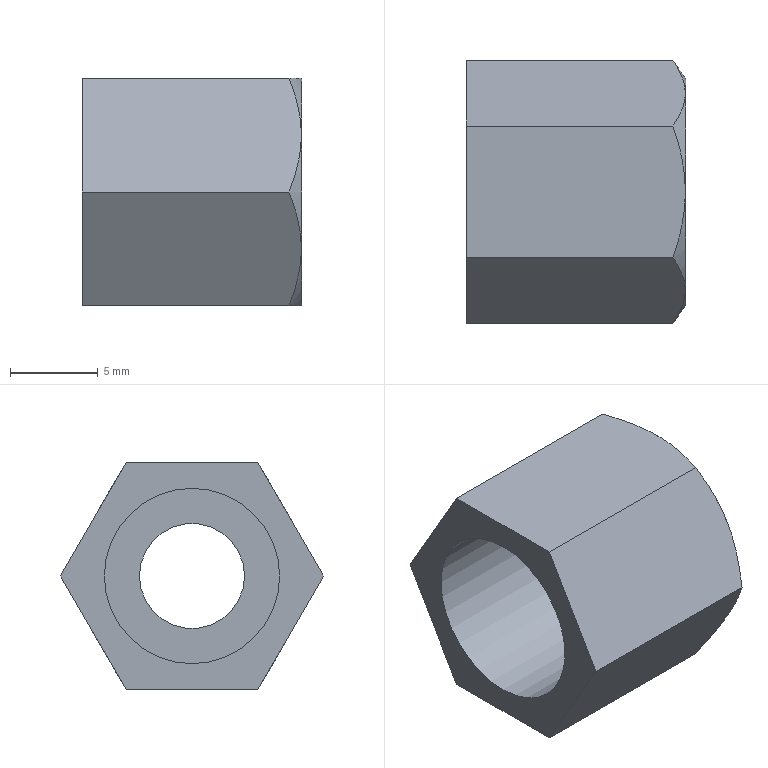Part | STEP file | 1-55.5 | 2 solids | 16 faces | box 12.5 x 15.011 x 13 mm | volume 1071 mm3 | plane 11 | cylinder 4 | cone 1 | commonest cylinder face diameters 6 x2 10 x2
STEP:
#1=CARTESIAN_POINT('',(0.,0.,0.));
#2=DIRECTION('',(0.,0.,1.));
#3=DIRECTION('',(1.,0.,0.));
#4=AXIS2_PLACEMENT_3D('',#1,#2,#3);
#5=CARTESIAN_POINT('',(0.,-3.753,6.5));
#6=VERTEX_POINT('',#5);
#7=CARTESIAN_POINT('',(0.,3.753,6.5));
#8=VERTEX_POINT('',#7);
#9=CARTESIAN_POINT('',(0.,-3.753,6.5));
#10=DIRECTION('',(0.,1.,0.));
#11=VECTOR('',#10,1.);
#12=LINE('',#9,#11);
#13=CARTESIAN_POINT('',(0.,0.,1.006));
#14=DIRECTION('',(-1.,0.,0.));
#15=DIRECTION('',(0.,0.,1.));
#16=AXIS2_PLACEMENT_3D('',#13,#14,#15);
#17=PLANE('',#16);
#18=CARTESIAN_POINT('',(5.494,-3.753));
#19=DIRECTION('',(0.,1.));
#20=VECTOR('',#19,1.);
#21=LINE('',#18,#20);
#22=(GEOMETRIC_REPRESENTATION_CONTEXT(2)PARAMETRIC_REPRESENTATION_CONTEXT()REPRESENTATION_CONTEXT('',''));
#23=DEFINITIONAL_REPRESENTATION('',(#21),#22);
#24=PCURVE('',#17,#23);
#25=CARTESIAN_POINT('',(6.25,0.,6.5));
#26=DIRECTION('',(0.,0.,-1.));
#27=DIRECTION('',(0.,1.,0.));
#28=AXIS2_PLACEMENT_3D('',#25,#26,#27);
#29=PLANE('',#28);
#30=CARTESIAN_POINT('',(-3.753,-6.25));
#31=DIRECTION('',(1.,0.));
#32=VECTOR('',#31,1.);
#33=LINE('',#30,#32);
#34=(GEOMETRIC_REPRESENTATION_CONTEXT(2)PARAMETRIC_REPRESENTATION_CONTEXT()REPRESENTATION_CONTEXT('',''));
#35=DEFINITIONAL_REPRESENTATION('',(#33),#34);
#36=PCURVE('',#29,#35);
#37=SURFACE_CURVE('',#12,(#24,#36),.PCURVE_S1.);
#38=EDGE_CURVE('',#6,#8,#37,.T.);
#39=ORIENTED_EDGE('',*,*,#38,.T.);
#40=CARTESIAN_POINT('',(0.,7.506,0.));
#41=VERTEX_POINT('',#40);
#42=CARTESIAN_POINT('',(0.,3.753,6.5));
#43=DIRECTION('',(0.,0.5,-0.866));
#44=VECTOR('',#43,1.);
#45=LINE('',#42,#44);
#46=CARTESIAN_POINT('',(5.494,3.753));
#47=DIRECTION('',(-0.866,0.5));
#48=VECTOR('',#47,1.);
#49=LINE('',#46,#48);
#50=(GEOMETRIC_REPRESENTATION_CONTEXT(2)PARAMETRIC_REPRESENTATION_CONTEXT()REPRESENTATION_CONTEXT('',''));
#51=DEFINITIONAL_REPRESENTATION('',(#49),#50);
#52=PCURVE('',#17,#51);
#53=CARTESIAN_POINT('',(6.25,5.629,3.25));
#54=DIRECTION('',(0.,-0.866,-0.5));
#55=DIRECTION('',(0.,0.5,-0.866));
#56=AXIS2_PLACEMENT_3D('',#53,#54,#55);
#57=PLANE('',#56);
#58=CARTESIAN_POINT('',(-3.753,-6.25));
#59=DIRECTION('',(1.,0.));
#60=VECTOR('',#59,1.);
#61=LINE('',#58,#60);
#62=(GEOMETRIC_REPRESENTATION_CONTEXT(2)PARAMETRIC_REPRESENTATION_CONTEXT()REPRESENTATION_CONTEXT('',''));
#63=DEFINITIONAL_REPRESENTATION('',(#61),#62);
#64=PCURVE('',#57,#63);
#65=SURFACE_CURVE('',#45,(#52,#64),.PCURVE_S1.);
#66=EDGE_CURVE('',#8,#41,#65,.T.);
#67=ORIENTED_EDGE('',*,*,#66,.T.);
#68=CARTESIAN_POINT('',(0.,3.753,-6.5));
#69=VERTEX_POINT('',#68);
#70=CARTESIAN_POINT('',(0.,7.506,0.));
#71=DIRECTION('',(0.,-0.5,-0.866));
#72=VECTOR('',#71,1.);
#73=LINE('',#70,#72);
#74=CARTESIAN_POINT('',(-1.006,7.506));
#75=DIRECTION('',(-0.866,-0.5));
#76=VECTOR('',#75,1.);
#77=LINE('',#74,#76);
#78=(GEOMETRIC_REPRESENTATION_CONTEXT(2)PARAMETRIC_REPRESENTATION_CONTEXT()REPRESENTATION_CONTEXT('',''));
#79=DEFINITIONAL_REPRESENTATION('',(#77),#78);
#80=PCURVE('',#17,#79);
#81=CARTESIAN_POINT('',(6.25,5.629,-3.25));
#82=DIRECTION('',(0.,-0.866,0.5));
#83=DIRECTION('',(0.,-0.5,-0.866));
#84=AXIS2_PLACEMENT_3D('',#81,#82,#83);
#85=PLANE('',#84);
#86=CARTESIAN_POINT('',(-3.753,-6.25));
#87=DIRECTION('',(1.,0.));
#88=VECTOR('',#87,1.);
#89=LINE('',#86,#88);
#90=(GEOMETRIC_REPRESENTATION_CONTEXT(2)PARAMETRIC_REPRESENTATION_CONTEXT()REPRESENTATION_CONTEXT('',''));
#91=DEFINITIONAL_REPRESENTATION('',(#89),#90);
#92=PCURVE('',#85,#91);
#93=SURFACE_CURVE('',#73,(#80,#92),.PCURVE_S1.);
#94=EDGE_CURVE('',#41,#69,#93,.T.);
#95=ORIENTED_EDGE('',*,*,#94,.T.);
#96=CARTESIAN_POINT('',(0.,-3.753,-6.5));
#97=VERTEX_POINT('',#96);
#98=CARTESIAN_POINT('',(0.,3.753,-6.5));
#99=DIRECTION('',(0.,-1.,0.));
#100=VECTOR('',#99,1.);
#101=LINE('',#98,#100);
#102=CARTESIAN_POINT('',(-7.506,3.753));
#103=DIRECTION('',(0.,-1.));
#104=VECTOR('',#103,1.);
#105=LINE('',#102,#104);
#106=(GEOMETRIC_REPRESENTATION_CONTEXT(2)PARAMETRIC_REPRESENTATION_CONTEXT()REPRESENTATION_CONTEXT('',''));
#107=DEFINITIONAL_REPRESENTATION('',(#105),#106);
#108=PCURVE('',#17,#107);
#109=CARTESIAN_POINT('',(6.25,0.,-6.5));
#110=DIRECTION('',(0.,0.,1.));
#111=DIRECTION('',(0.,-1.,0.));
#112=AXIS2_PLACEMENT_3D('',#109,#110,#111);
#113=PLANE('',#112);
#114=CARTESIAN_POINT('',(-3.753,-6.25));
#115=DIRECTION('',(1.,0.));
#116=VECTOR('',#115,1.);
#117=LINE('',#114,#116);
#118=(GEOMETRIC_REPRESENTATION_CONTEXT(2)PARAMETRIC_REPRESENTATION_CONTEXT()REPRESENTATION_CONTEXT('',''));
#119=DEFINITIONAL_REPRESENTATION('',(#117),#118);
#120=PCURVE('',#113,#119);
#121=SURFACE_CURVE('',#101,(#108,#120),.PCURVE_S1.);
#122=EDGE_CURVE('',#69,#97,#121,.T.);
#123=ORIENTED_EDGE('',*,*,#122,.T.);
#124=CARTESIAN_POINT('',(0.,-7.506,0.));
#125=VERTEX_POINT('',#124);
#126=CARTESIAN_POINT('',(0.,-3.753,-6.5));
#127=DIRECTION('',(0.,-0.5,0.866));
#128=VECTOR('',#127,1.);
#129=LINE('',#126,#128);
#130=CARTESIAN_POINT('',(-7.506,-3.753));
#131=DIRECTION('',(0.866,-0.5));
#132=VECTOR('',#131,1.);
#133=LINE('',#130,#132);
#134=(GEOMETRIC_REPRESENTATION_CONTEXT(2)PARAMETRIC_REPRESENTATION_CONTEXT()REPRESENTATION_CONTEXT('',''));
#135=DEFINITIONAL_REPRESENTATION('',(#133),#134);
#136=PCURVE('',#17,#135);
#137=CARTESIAN_POINT('',(6.25,-5.629,-3.25));
#138=DIRECTION('',(0.,0.866,0.5));
#139=DIRECTION('',(0.,-0.5,0.866));
#140=AXIS2_PLACEMENT_3D('',#137,#138,#139);
#141=PLANE('',#140);
#142=CARTESIAN_POINT('',(-3.753,-6.25));
#143=DIRECTION('',(1.,0.));
#144=VECTOR('',#143,1.);
#145=LINE('',#142,#144);
#146=(GEOMETRIC_REPRESENTATION_CONTEXT(2)PARAMETRIC_REPRESENTATION_CONTEXT()REPRESENTATION_CONTEXT('',''));
#147=DEFINITIONAL_REPRESENTATION('',(#145),#146);
#148=PCURVE('',#141,#147);
#149=SURFACE_CURVE('',#129,(#136,#148),.PCURVE_S1.);
#150=EDGE_CURVE('',#97,#125,#149,.T.);
#151=ORIENTED_EDGE('',*,*,#150,.T.);
#152=CARTESIAN_POINT('',(0.,-7.506,0.));
#153=DIRECTION('',(0.,0.5,0.866));
#154=VECTOR('',#153,1.);
#155=LINE('',#152,#154);
#156=CARTESIAN_POINT('',(-1.006,-7.506));
#157=DIRECTION('',(0.866,0.5));
#158=VECTOR('',#157,1.);
#159=LINE('',#156,#158);
#160=(GEOMETRIC_REPRESENTATION_CONTEXT(2)PARAMETRIC_REPRESENTATION_CONTEXT()REPRESENTATION_CONTEXT('',''));
#161=DEFINITIONAL_REPRESENTATION('',(#159),#160);
#162=PCURVE('',#17,#161);
#163=CARTESIAN_POINT('',(6.25,-5.629,3.25));
#164=DIRECTION('',(0.,0.866,-0.5));
#165=DIRECTION('',(0.,0.5,0.866));
#166=AXIS2_PLACEMENT_3D('',#163,#164,#165);
#167=PLANE('',#166);
#168=CARTESIAN_POINT('',(-3.753,-6.25));
#169=DIRECTION('',(1.,0.));
#170=VECTOR('',#169,1.);
#171=LINE('',#168,#170);
#172=(GEOMETRIC_REPRESENTATION_CONTEXT(2)PARAMETRIC_REPRESENTATION_CONTEXT()REPRESENTATION_CONTEXT('',''));
#173=DEFINITIONAL_REPRESENTATION('',(#171),#172);
#174=PCURVE('',#167,#173);
#175=SURFACE_CURVE('',#155,(#162,#174),.PCURVE_S1.);
#176=EDGE_CURVE('',#125,#6,#175,.T.);
#177=ORIENTED_EDGE('',*,*,#176,.T.);
#178=EDGE_LOOP('',(#39,#67,#95,#123,#151,#177));
#179=FACE_BOUND('',#178,.T.);
#180=CARTESIAN_POINT('',(0.,5.,0.));
#181=VERTEX_POINT('',#180);
#182=CARTESIAN_POINT('',(0.,0.,0.));
#183=DIRECTION('',(1.,0.,0.));
#184=DIRECTION('',(0.,1.,0.));
#185=AXIS2_PLACEMENT_3D('',#182,#183,#184);
#186=CIRCLE('',#185,5.);
#187=CARTESIAN_POINT('',(-1.006,5.));
#188=CARTESIAN_POINT('',(7.655,5.));
#189=CARTESIAN_POINT('',(3.325,-2.5));
#190=CARTESIAN_POINT('',(-1.006,-10.));
#191=CARTESIAN_POINT('',(-5.336,-2.5));
#192=CARTESIAN_POINT('',(-9.666,5.));
#193=CARTESIAN_POINT('',(-1.006,5.));
#194=(BOUNDED_CURVE()B_SPLINE_CURVE(2,(#187,#188,#189,#190,#191,#192,#193),.UNSPECIFIED.,.T.,.F.)B_SPLINE_CURVE_WITH_KNOTS((1,2,2,2,2,1),(-2.094,0.,2.094,4.189,6.283,8.378),.UNSPECIFIED.)CURVE()GEOMETRIC_REPRESENTATION_ITEM()RATIONAL_B_SPLINE_CURVE((1.,0.5,1.,0.5,1.,0.5,1.))REPRESENTATION_ITEM(''));
#195=(GEOMETRIC_REPRESENTATION_CONTEXT(2)PARAMETRIC_REPRESENTATION_CONTEXT()REPRESENTATION_CONTEXT('',''));
#196=DEFINITIONAL_REPRESENTATION('',(#194),#195);
#197=PCURVE('',#17,#196);
#198=CARTESIAN_POINT('',(0.,0.,0.));
#199=DIRECTION('',(1.,0.,0.));
#200=DIRECTION('',(0.,1.,0.));
#201=AXIS2_PLACEMENT_3D('',#198,#199,#200);
#202=CYLINDRICAL_SURFACE('',#201,5.);
#203=CARTESIAN_POINT('',(0.,0.));
#204=DIRECTION('',(1.,0.));
#205=VECTOR('',#204,1.);
#206=LINE('',#203,#205);
#207=(GEOMETRIC_REPRESENTATION_CONTEXT(2)PARAMETRIC_REPRESENTATION_CONTEXT()REPRESENTATION_CONTEXT('',''));
#208=DEFINITIONAL_REPRESENTATION('',(#206),#207);
#209=PCURVE('',#202,#208);
#210=SURFACE_CURVE('',#186,(#197,#209),.PCURVE_S1.);
#211=EDGE_CURVE('',#181,#181,#210,.T.);
#212=ORIENTED_EDGE('',*,*,#211,.T.);
#213=EDGE_LOOP('',(#212));
#214=FACE_BOUND('',#213,.T.);
#215=ADVANCED_FACE('',(#179,#214),#17,.T.);
#216=ORIENTED_EDGE('',*,*,#211,.T.);
#217=CARTESIAN_POINT('',(10.,5.,0.));
#218=VERTEX_POINT('',#217);
#219=CARTESIAN_POINT('',(0.,5.,0.));
#220=DIRECTION('',(1.,0.,0.));
#221=VECTOR('',#220,1.);
#222=LINE('',#219,#221);
#223=CARTESIAN_POINT('',(6.283,0.));
#224=DIRECTION('',(0.,1.));
#225=VECTOR('',#224,1.);
#226=LINE('',#223,#225);
#227=(GEOMETRIC_REPRESENTATION_CONTEXT(2)PARAMETRIC_REPRESENTATION_CONTEXT()REPRESENTATION_CONTEXT('',''));
#228=DEFINITIONAL_REPRESENTATION('',(#226),#227);
#229=PCURVE('',#202,#228);
#230=CARTESIAN_POINT('',(0.,0.));
#231=DIRECTION('',(0.,1.));
#232=VECTOR('',#231,1.);
#233=LINE('',#230,#232);
#234=(GEOMETRIC_REPRESENTATION_CONTEXT(2)PARAMETRIC_REPRESENTATION_CONTEXT()REPRESENTATION_CONTEXT('',''));
#235=DEFINITIONAL_REPRESENTATION('',(#233),#234);
#236=PCURVE('',#202,#235);
#237=SEAM_CURVE('',#222,(#229,#236),.PCURVE_S1.);
#238=EDGE_CURVE('',#181,#218,#237,.T.);
#239=ORIENTED_EDGE('',*,*,#238,.T.);
#240=CARTESIAN_POINT('',(10.,0.,0.));
#241=DIRECTION('',(1.,0.,0.));
#242=DIRECTION('',(0.,1.,0.));
#243=AXIS2_PLACEMENT_3D('',#240,#241,#242);
#244=CIRCLE('',#243,5.);
#245=CARTESIAN_POINT('',(0.,10.));
#246=DIRECTION('',(1.,0.));
#247=VECTOR('',#246,1.);
#248=LINE('',#245,#247);
#249=(GEOMETRIC_REPRESENTATION_CONTEXT(2)PARAMETRIC_REPRESENTATION_CONTEXT()REPRESENTATION_CONTEXT('',''));
#250=DEFINITIONAL_REPRESENTATION('',(#248),#249);
#251=PCURVE('',#202,#250);
#252=CARTESIAN_POINT('',(10.,-1.34,0.));
#253=DIRECTION('',(1.,0.,0.));
#254=DIRECTION('',(0.,0.,-1.));
#255=AXIS2_PLACEMENT_3D('',#252,#253,#254);
#256=PLANE('',#255);
#257=CARTESIAN_POINT('',(0.,1.34));
#258=DIRECTION('',(0.,1.));
#259=AXIS2_PLACEMENT_2D('',#257,#258);
#260=CIRCLE('',#259,5.);
#261=(GEOMETRIC_REPRESENTATION_CONTEXT(2)PARAMETRIC_REPRESENTATION_CONTEXT()REPRESENTATION_CONTEXT('',''));
#262=DEFINITIONAL_REPRESENTATION('',(#260),#261);
#263=PCURVE('',#256,#262);
#264=SURFACE_CURVE('',#244,(#251,#263),.PCURVE_S1.);
#265=EDGE_CURVE('',#218,#218,#264,.T.);
#266=ORIENTED_EDGE('',*,*,#265,.F.);
#267=ORIENTED_EDGE('',*,*,#238,.F.);
#268=EDGE_LOOP('',(#216,#239,#266,#267));
#269=FACE_BOUND('',#268,.F.);
#270=ADVANCED_FACE('',(#269),#202,.F.);
#271=ORIENTED_EDGE('',*,*,#265,.T.);
#272=EDGE_LOOP('',(#271));
#273=FACE_BOUND('',#272,.F.);
#274=CARTESIAN_POINT('',(10.,3.,0.));
#275=VERTEX_POINT('',#274);
#276=CARTESIAN_POINT('',(10.,0.,0.));
#277=DIRECTION('',(-1.,0.,0.));
#278=DIRECTION('',(0.,1.,0.));
#279=AXIS2_PLACEMENT_3D('',#276,#277,#278);
#280=CIRCLE('',#279,3.);
#281=CARTESIAN_POINT('',(0.,4.34));
#282=CARTESIAN_POINT('',(5.196,4.34));
#283=CARTESIAN_POINT('',(2.598,-0.1603));
#284=CARTESIAN_POINT('',(0.,-4.66));
#285=CARTESIAN_POINT('',(-2.598,-0.1603));
#286=CARTESIAN_POINT('',(-5.196,4.34));
#287=CARTESIAN_POINT('',(0.,4.34));
#288=(BOUNDED_CURVE()B_SPLINE_CURVE(2,(#281,#282,#283,#284,#285,#286,#287),.UNSPECIFIED.,.T.,.F.)B_SPLINE_CURVE_WITH_KNOTS((1,2,2,2,2,1),(-2.094,0.,2.094,4.189,6.283,8.378),.UNSPECIFIED.)CURVE()GEOMETRIC_REPRESENTATION_ITEM()RATIONAL_B_SPLINE_CURVE((1.,0.5,1.,0.5,1.,0.5,1.))REPRESENTATION_ITEM(''));
#289=(GEOMETRIC_REPRESENTATION_CONTEXT(2)PARAMETRIC_REPRESENTATION_CONTEXT()REPRESENTATION_CONTEXT('',''));
#290=DEFINITIONAL_REPRESENTATION('',(#288),#289);
#291=PCURVE('',#256,#290);
#292=CARTESIAN_POINT('',(0.,0.,0.));
#293=DIRECTION('',(1.,0.,0.));
#294=DIRECTION('',(0.,1.,0.));
#295=AXIS2_PLACEMENT_3D('',#292,#293,#294);
#296=CYLINDRICAL_SURFACE('',#295,3.);
#297=CARTESIAN_POINT('',(6.283,10.));
#298=DIRECTION('',(-1.,0.));
#299=VECTOR('',#298,1.);
#300=LINE('',#297,#299);
#301=(GEOMETRIC_REPRESENTATION_CONTEXT(2)PARAMETRIC_REPRESENTATION_CONTEXT()REPRESENTATION_CONTEXT('',''));
#302=DEFINITIONAL_REPRESENTATION('',(#300),#301);
#303=PCURVE('',#296,#302);
#304=SURFACE_CURVE('',#280,(#291,#303),.PCURVE_S1.);
#305=EDGE_CURVE('',#275,#275,#304,.T.);
#306=ORIENTED_EDGE('',*,*,#305,.T.);
#307=EDGE_LOOP('',(#306));
#308=FACE_BOUND('',#307,.F.);
#309=ADVANCED_FACE('',(#273,#308),#256,.F.);
#310=CARTESIAN_POINT('',(12.5,3.,0.));
#311=VERTEX_POINT('',#310);
#312=CARTESIAN_POINT('',(12.5,0.,0.));
#313=DIRECTION('',(1.,0.,0.));
#314=DIRECTION('',(0.,1.,0.));
#315=AXIS2_PLACEMENT_3D('',#312,#313,#314);
#316=CIRCLE('',#315,3.);
#317=CARTESIAN_POINT('',(0.,12.5));
#318=DIRECTION('',(1.,0.));
#319=VECTOR('',#318,1.);
#320=LINE('',#317,#319);
#321=(GEOMETRIC_REPRESENTATION_CONTEXT(2)PARAMETRIC_REPRESENTATION_CONTEXT()REPRESENTATION_CONTEXT('',''));
#322=DEFINITIONAL_REPRESENTATION('',(#320),#321);
#323=PCURVE('',#296,#322);
#324=CARTESIAN_POINT('',(12.5,0.,1.006));
#325=DIRECTION('',(-1.,0.,0.));
#326=DIRECTION('',(0.,0.,1.));
#327=AXIS2_PLACEMENT_3D('',#324,#325,#326);
#328=PLANE('',#327);
#329=CARTESIAN_POINT('',(-1.006,3.));
#330=CARTESIAN_POINT('',(4.191,3.));
#331=CARTESIAN_POINT('',(1.593,-1.5));
#332=CARTESIAN_POINT('',(-1.006,-6.));
#333=CARTESIAN_POINT('',(-3.604,-1.5));
#334=CARTESIAN_POINT('',(-6.202,3.));
#335=CARTESIAN_POINT('',(-1.006,3.));
#336=(BOUNDED_CURVE()B_SPLINE_CURVE(2,(#329,#330,#331,#332,#333,#334,#335),.UNSPECIFIED.,.T.,.F.)B_SPLINE_CURVE_WITH_KNOTS((1,2,2,2,2,1),(-2.094,0.,2.094,4.189,6.283,8.378),.UNSPECIFIED.)CURVE()GEOMETRIC_REPRESENTATION_ITEM()RATIONAL_B_SPLINE_CURVE((1.,0.5,1.,0.5,1.,0.5,1.))REPRESENTATION_ITEM(''));
#337=(GEOMETRIC_REPRESENTATION_CONTEXT(2)PARAMETRIC_REPRESENTATION_CONTEXT()REPRESENTATION_CONTEXT('',''));
#338=DEFINITIONAL_REPRESENTATION('',(#336),#337);
#339=PCURVE('',#328,#338);
#340=SURFACE_CURVE('',#316,(#323,#339),.PCURVE_S1.);
#341=EDGE_CURVE('',#311,#311,#340,.T.);
#342=ORIENTED_EDGE('',*,*,#341,.F.);
#343=CARTESIAN_POINT('',(10.,3.,0.));
#344=DIRECTION('',(1.,0.,0.));
#345=VECTOR('',#344,1.);
#346=LINE('',#343,#345);
#347=CARTESIAN_POINT('',(0.,10.));
#348=DIRECTION('',(0.,1.));
#349=VECTOR('',#348,1.);
#350=LINE('',#347,#349);
#351=(GEOMETRIC_REPRESENTATION_CONTEXT(2)PARAMETRIC_REPRESENTATION_CONTEXT()REPRESENTATION_CONTEXT('',''));
#352=DEFINITIONAL_REPRESENTATION('',(#350),#351);
#353=PCURVE('',#296,#352);
#354=CARTESIAN_POINT('',(6.283,10.));
#355=DIRECTION('',(0.,1.));
#356=VECTOR('',#355,1.);
#357=LINE('',#354,#356);
#358=(GEOMETRIC_REPRESENTATION_CONTEXT(2)PARAMETRIC_REPRESENTATION_CONTEXT()REPRESENTATION_CONTEXT('',''));
#359=DEFINITIONAL_REPRESENTATION('',(#357),#358);
#360=PCURVE('',#296,#359);
#361=SEAM_CURVE('',#346,(#353,#360),.PCURVE_S1.);
#362=EDGE_CURVE('',#275,#311,#361,.T.);
#363=ORIENTED_EDGE('',*,*,#362,.F.);
#364=ORIENTED_EDGE('',*,*,#305,.F.);
#365=ORIENTED_EDGE('',*,*,#362,.T.);
#366=EDGE_LOOP('',(#342,#363,#364,#365));
#367=FACE_BOUND('',#366,.F.);
#368=ADVANCED_FACE('',(#367),#296,.F.);
#369=ORIENTED_EDGE('',*,*,#38,.T.);
#370=CARTESIAN_POINT('',(11.786,3.753,6.5));
#371=VERTEX_POINT('',#370);
#372=CARTESIAN_POINT('',(0.,3.753,6.5));
#373=DIRECTION('',(1.,0.,0.));
#374=VECTOR('',#373,1.);
#375=LINE('',#372,#374);
#376=CARTESIAN_POINT('',(3.753,-6.25));
#377=DIRECTION('',(0.,1.));
#378=VECTOR('',#377,1.);
#379=LINE('',#376,#378);
#380=(GEOMETRIC_REPRESENTATION_CONTEXT(2)PARAMETRIC_REPRESENTATION_CONTEXT()REPRESENTATION_CONTEXT('',''));
#381=DEFINITIONAL_REPRESENTATION('',(#379),#380);
#382=PCURVE('',#29,#381);
#383=CARTESIAN_POINT('',(-3.753,-6.25));
#384=DIRECTION('',(0.,1.));
#385=VECTOR('',#384,1.);
#386=LINE('',#383,#385);
#387=(GEOMETRIC_REPRESENTATION_CONTEXT(2)PARAMETRIC_REPRESENTATION_CONTEXT()REPRESENTATION_CONTEXT('',''));
#388=DEFINITIONAL_REPRESENTATION('',(#386),#387);
#389=PCURVE('',#57,#388);
#390=SURFACE_CURVE('',#375,(#382,#389),.PCURVE_S1.);
#391=EDGE_CURVE('',#8,#371,#390,.T.);
#392=ORIENTED_EDGE('',*,*,#391,.T.);
#393=CARTESIAN_POINT('',(12.485,0.,6.5));
#394=VERTEX_POINT('',#393);
#395=CARTESIAN_POINT('',(11.786,3.753,6.5));
#396=CARTESIAN_POINT('',(12.485,1.742,6.5));
#397=CARTESIAN_POINT('',(12.485,0.,6.5));
#398=(BOUNDED_CURVE()B_SPLINE_CURVE(2,(#395,#396,#397),.UNSPECIFIED.,.F.,.F.)B_SPLINE_CURVE_WITH_KNOTS((3,3),(0.,1.),.PIECEWISE_BEZIER_KNOTS.)CURVE()GEOMETRIC_REPRESENTATION_ITEM()RATIONAL_B_SPLINE_CURVE((1.502,1.619,1.619))REPRESENTATION_ITEM(''));
#399=CARTESIAN_POINT('',(3.753,5.536));
#400=CARTESIAN_POINT('',(1.742,6.235));
#401=CARTESIAN_POINT('',(0.,6.235));
#402=(BOUNDED_CURVE()B_SPLINE_CURVE(2,(#399,#400,#401),.UNSPECIFIED.,.F.,.F.)B_SPLINE_CURVE_WITH_KNOTS((3,3),(0.,1.),.PIECEWISE_BEZIER_KNOTS.)CURVE()GEOMETRIC_REPRESENTATION_ITEM()RATIONAL_B_SPLINE_CURVE((1.502,1.619,1.619))REPRESENTATION_ITEM(''));
#403=(GEOMETRIC_REPRESENTATION_CONTEXT(2)PARAMETRIC_REPRESENTATION_CONTEXT()REPRESENTATION_CONTEXT('',''));
#404=DEFINITIONAL_REPRESENTATION('',(#402),#403);
#405=PCURVE('',#29,#404);
#406=CARTESIAN_POINT('',(12.5,0.,0.));
#407=DIRECTION('',(-1.,0.,0.));
#408=DIRECTION('',(0.,0.,1.));
#409=AXIS2_PLACEMENT_3D('',#406,#407,#408);
#410=CONICAL_SURFACE('',#409,6.478,0.9631);
#411=CARTESIAN_POINT('',(0.5236,0.7145));
#412=CARTESIAN_POINT('',(0.516,0.6916));
#413=CARTESIAN_POINT('',(0.5008,0.6473));
#414=CARTESIAN_POINT('',(0.4779,0.5848));
#415=CARTESIAN_POINT('',(0.4548,0.5261));
#416=CARTESIAN_POINT('',(0.4317,0.471));
#417=CARTESIAN_POINT('',(0.4084,0.4195));
#418=CARTESIAN_POINT('',(0.3849,0.3714));
#419=CARTESIAN_POINT('',(0.3614,0.3267));
#420=CARTESIAN_POINT('',(0.3378,0.2853));
#421=CARTESIAN_POINT('',(0.3141,0.2471));
#422=CARTESIAN_POINT('',(0.2903,0.2119));
#423=CARTESIAN_POINT('',(0.2664,0.1798));
#424=CARTESIAN_POINT('',(0.2424,0.1507));
#425=CARTESIAN_POINT('',(0.2184,0.1245));
#426=CARTESIAN_POINT('',(0.1943,0.1013));
#427=CARTESIAN_POINT('',(0.1701,0.0808));
#428=CARTESIAN_POINT('',(0.1459,0.06314));
#429=CARTESIAN_POINT('',(0.1217,0.04826));
#430=CARTESIAN_POINT('',(0.09736,0.03611));
#431=CARTESIAN_POINT('',(0.07305,0.02669));
#432=CARTESIAN_POINT('',(0.04871,0.01998));
#433=CARTESIAN_POINT('',(0.02436,0.01595));
#434=CARTESIAN_POINT('',(0.00812,0.01506));
#435=CARTESIAN_POINT('',(0.,0.01506));
#436=B_SPLINE_CURVE_WITH_KNOTS('',3,(#411,#412,#413,#414,#415,#416,#417,#418,#419,#420,#421,#422,#423,#424,#425,#426,#427,#428,#429,#430,#431,#432,#433,#434,#435),.UNSPECIFIED.,.F.,.F.,(4,1,1,1,1,1,1,1,1,1,1,1,1,1,1,1,1,1,1,1,1,1,4),(0.,0.04545,0.09091,0.1364,0.1818,0.2273,0.2727,0.3182,0.3636,0.4091,0.4545,0.5,0.5455,0.5909,0.6364,0.6818,0.7273,0.7727,0.8182,0.8636,0.9091,0.9545,1.),.QUASI_UNIFORM_KNOTS.);
#437=(GEOMETRIC_REPRESENTATION_CONTEXT(2)PARAMETRIC_REPRESENTATION_CONTEXT()REPRESENTATION_CONTEXT('',''));
#438=DEFINITIONAL_REPRESENTATION('',(#436),#437);
#439=PCURVE('',#410,#438);
#440=SURFACE_CURVE('',#398,(#405,#439),.PCURVE_S1.);
#441=EDGE_CURVE('',#371,#394,#440,.T.);
#442=ORIENTED_EDGE('',*,*,#441,.T.);
#443=CARTESIAN_POINT('',(11.786,-3.753,6.5));
#444=VERTEX_POINT('',#443);
#445=CARTESIAN_POINT('',(12.485,0.,6.5));
#446=CARTESIAN_POINT('',(12.485,-1.742,6.5));
#447=CARTESIAN_POINT('',(11.786,-3.753,6.5));
#448=(BOUNDED_CURVE()B_SPLINE_CURVE(2,(#445,#446,#447),.UNSPECIFIED.,.F.,.F.)B_SPLINE_CURVE_WITH_KNOTS((3,3),(0.,1.),.PIECEWISE_BEZIER_KNOTS.)CURVE()GEOMETRIC_REPRESENTATION_ITEM()RATIONAL_B_SPLINE_CURVE((1.619,1.619,1.502))REPRESENTATION_ITEM(''));
#449=CARTESIAN_POINT('',(0.,6.235));
#450=CARTESIAN_POINT('',(-1.742,6.235));
#451=CARTESIAN_POINT('',(-3.753,5.536));
#452=(BOUNDED_CURVE()B_SPLINE_CURVE(2,(#449,#450,#451),.UNSPECIFIED.,.F.,.F.)B_SPLINE_CURVE_WITH_KNOTS((3,3),(0.,1.),.PIECEWISE_BEZIER_KNOTS.)CURVE()GEOMETRIC_REPRESENTATION_ITEM()RATIONAL_B_SPLINE_CURVE((1.619,1.619,1.502))REPRESENTATION_ITEM(''));
#453=(GEOMETRIC_REPRESENTATION_CONTEXT(2)PARAMETRIC_REPRESENTATION_CONTEXT()REPRESENTATION_CONTEXT('',''));
#454=DEFINITIONAL_REPRESENTATION('',(#452),#453);
#455=PCURVE('',#29,#454);
#456=CARTESIAN_POINT('',(6.283,0.01506));
#457=CARTESIAN_POINT('',(6.275,0.01506));
#458=CARTESIAN_POINT('',(6.259,0.01595));
#459=CARTESIAN_POINT('',(6.234,0.01998));
#460=CARTESIAN_POINT('',(6.21,0.02669));
#461=CARTESIAN_POINT('',(6.186,0.03611));
#462=CARTESIAN_POINT('',(6.162,0.04826));
#463=CARTESIAN_POINT('',(6.137,0.06314));
#464=CARTESIAN_POINT('',(6.113,0.0808));
#465=CARTESIAN_POINT('',(6.089,0.1013));
#466=CARTESIAN_POINT('',(6.065,0.1245));
#467=CARTESIAN_POINT('',(6.041,0.1507));
#468=CARTESIAN_POINT('',(6.017,0.1798));
#469=CARTESIAN_POINT('',(5.993,0.2119));
#470=CARTESIAN_POINT('',(5.969,0.2471));
#471=CARTESIAN_POINT('',(5.945,0.2853));
#472=CARTESIAN_POINT('',(5.922,0.3267));
#473=CARTESIAN_POINT('',(5.898,0.3714));
#474=CARTESIAN_POINT('',(5.875,0.4195));
#475=CARTESIAN_POINT('',(5.852,0.471));
#476=CARTESIAN_POINT('',(5.828,0.5261));
#477=CARTESIAN_POINT('',(5.805,0.5848));
#478=CARTESIAN_POINT('',(5.782,0.6473));
#479=CARTESIAN_POINT('',(5.767,0.6916));
#480=CARTESIAN_POINT('',(5.76,0.7145));
#481=B_SPLINE_CURVE_WITH_KNOTS('',3,(#456,#457,#458,#459,#460,#461,#462,#463,#464,#465,#466,#467,#468,#469,#470,#471,#472,#473,#474,#475,#476,#477,#478,#479,#480),.UNSPECIFIED.,.F.,.F.,(4,1,1,1,1,1,1,1,1,1,1,1,1,1,1,1,1,1,1,1,1,1,4),(0.,0.04545,0.09091,0.1364,0.1818,0.2273,0.2727,0.3182,0.3636,0.4091,0.4545,0.5,0.5455,0.5909,0.6364,0.6818,0.7273,0.7727,0.8182,0.8636,0.9091,0.9545,1.),.QUASI_UNIFORM_KNOTS.);
#482=(GEOMETRIC_REPRESENTATION_CONTEXT(2)PARAMETRIC_REPRESENTATION_CONTEXT()REPRESENTATION_CONTEXT('',''));
#483=DEFINITIONAL_REPRESENTATION('',(#481),#482);
#484=PCURVE('',#410,#483);
#485=SURFACE_CURVE('',#448,(#455,#484),.PCURVE_S1.);
#486=EDGE_CURVE('',#394,#444,#485,.T.);
#487=ORIENTED_EDGE('',*,*,#486,.T.);
#488=CARTESIAN_POINT('',(0.,-3.753,6.5));
#489=DIRECTION('',(1.,0.,0.));
#490=VECTOR('',#489,1.);
#491=LINE('',#488,#490);
#492=CARTESIAN_POINT('',(-3.753,-6.25));
#493=DIRECTION('',(0.,1.));
#494=VECTOR('',#493,1.);
#495=LINE('',#492,#494);
#496=(GEOMETRIC_REPRESENTATION_CONTEXT(2)PARAMETRIC_REPRESENTATION_CONTEXT()REPRESENTATION_CONTEXT('',''));
#497=DEFINITIONAL_REPRESENTATION('',(#495),#496);
#498=PCURVE('',#29,#497);
#499=CARTESIAN_POINT('',(3.753,-6.25));
#500=DIRECTION('',(0.,1.));
#501=VECTOR('',#500,1.);
#502=LINE('',#499,#501);
#503=(GEOMETRIC_REPRESENTATION_CONTEXT(2)PARAMETRIC_REPRESENTATION_CONTEXT()REPRESENTATION_CONTEXT('',''));
#504=DEFINITIONAL_REPRESENTATION('',(#502),#503);
#505=PCURVE('',#167,#504);
#506=SURFACE_CURVE('',#491,(#498,#505),.PCURVE_S1.);
#507=EDGE_CURVE('',#6,#444,#506,.T.);
#508=ORIENTED_EDGE('',*,*,#507,.F.);
#509=EDGE_LOOP('',(#369,#392,#442,#487,#508));
#510=FACE_BOUND('',#509,.F.);
#511=ADVANCED_FACE('',(#510),#29,.F.);
#512=ORIENTED_EDGE('',*,*,#66,.T.);
#513=CARTESIAN_POINT('',(11.786,7.506,0.));
#514=VERTEX_POINT('',#513);
#515=CARTESIAN_POINT('',(0.,7.506,0.));
#516=DIRECTION('',(1.,0.,0.));
#517=VECTOR('',#516,1.);
#518=LINE('',#515,#517);
#519=CARTESIAN_POINT('',(3.753,-6.25));
#520=DIRECTION('',(0.,1.));
#521=VECTOR('',#520,1.);
#522=LINE('',#519,#521);
#523=(GEOMETRIC_REPRESENTATION_CONTEXT(2)PARAMETRIC_REPRESENTATION_CONTEXT()REPRESENTATION_CONTEXT('',''));
#524=DEFINITIONAL_REPRESENTATION('',(#522),#523);
#525=PCURVE('',#57,#524);
#526=CARTESIAN_POINT('',(-3.753,-6.25));
#527=DIRECTION('',(0.,1.));
#528=VECTOR('',#527,1.);
#529=LINE('',#526,#528);
#530=(GEOMETRIC_REPRESENTATION_CONTEXT(2)PARAMETRIC_REPRESENTATION_CONTEXT()REPRESENTATION_CONTEXT('',''));
#531=DEFINITIONAL_REPRESENTATION('',(#529),#530);
#532=PCURVE('',#85,#531);
#533=SURFACE_CURVE('',#518,(#525,#532),.PCURVE_S1.);
#534=EDGE_CURVE('',#41,#514,#533,.T.);
#535=ORIENTED_EDGE('',*,*,#534,.T.);
#536=CARTESIAN_POINT('',(11.786,7.506,0.));
#537=CARTESIAN_POINT('',(13.091,5.629,3.25));
#538=CARTESIAN_POINT('',(11.786,3.753,6.5));
#539=(BOUNDED_CURVE()B_SPLINE_CURVE(2,(#536,#537,#538),.UNSPECIFIED.,.F.,.F.)B_SPLINE_CURVE_WITH_KNOTS((3,3),(0.,1.),.PIECEWISE_BEZIER_KNOTS.)CURVE()GEOMETRIC_REPRESENTATION_ITEM()RATIONAL_B_SPLINE_CURVE((1.502,1.735,1.502))REPRESENTATION_ITEM(''));
#540=CARTESIAN_POINT('',(3.753,5.536));
#541=CARTESIAN_POINT('',(0.,6.841));
#542=CARTESIAN_POINT('',(-3.753,5.536));
#543=(BOUNDED_CURVE()B_SPLINE_CURVE(2,(#540,#541,#542),.UNSPECIFIED.,.F.,.F.)B_SPLINE_CURVE_WITH_KNOTS((3,3),(0.,1.),.PIECEWISE_BEZIER_KNOTS.)CURVE()GEOMETRIC_REPRESENTATION_ITEM()RATIONAL_B_SPLINE_CURVE((1.502,1.735,1.502))REPRESENTATION_ITEM(''));
#544=(GEOMETRIC_REPRESENTATION_CONTEXT(2)PARAMETRIC_REPRESENTATION_CONTEXT()REPRESENTATION_CONTEXT('',''));
#545=DEFINITIONAL_REPRESENTATION('',(#543),#544);
#546=PCURVE('',#57,#545);
#547=CARTESIAN_POINT('',(1.571,0.7145));
#548=CARTESIAN_POINT('',(1.556,0.6688));
#549=CARTESIAN_POINT('',(1.525,0.5829));
#550=CARTESIAN_POINT('',(1.479,0.4692));
#551=CARTESIAN_POINT('',(1.432,0.3698));
#552=CARTESIAN_POINT('',(1.385,0.2837));
#553=CARTESIAN_POINT('',(1.338,0.2104));
#554=CARTESIAN_POINT('',(1.29,0.1493));
#555=CARTESIAN_POINT('',(1.241,0.09983));
#556=CARTESIAN_POINT('',(1.193,0.06176));
#557=CARTESIAN_POINT('',(1.145,0.03476));
#558=CARTESIAN_POINT('',(1.096,0.01863));
#559=CARTESIAN_POINT('',(1.047,0.01327));
#560=CARTESIAN_POINT('',(0.9985,0.01863));
#561=CARTESIAN_POINT('',(0.9498,0.03476));
#562=CARTESIAN_POINT('',(0.9013,0.06176));
#563=CARTESIAN_POINT('',(0.8529,0.09983));
#564=CARTESIAN_POINT('',(0.8048,0.1493));
#565=CARTESIAN_POINT('',(0.7569,0.2104));
#566=CARTESIAN_POINT('',(0.7094,0.2837));
#567=CARTESIAN_POINT('',(0.6622,0.3698));
#568=CARTESIAN_POINT('',(0.6155,0.4692));
#569=CARTESIAN_POINT('',(0.5692,0.5829));
#570=CARTESIAN_POINT('',(0.5388,0.6688));
#571=CARTESIAN_POINT('',(0.5236,0.7145));
#572=B_SPLINE_CURVE_WITH_KNOTS('',3,(#547,#548,#549,#550,#551,#552,#553,#554,#555,#556,#557,#558,#559,#560,#561,#562,#563,#564,#565,#566,#567,#568,#569,#570,#571),.UNSPECIFIED.,.F.,.F.,(4,1,1,1,1,1,1,1,1,1,1,1,1,1,1,1,1,1,1,1,1,1,4),(0.,0.04545,0.09091,0.1364,0.1818,0.2273,0.2727,0.3182,0.3636,0.4091,0.4545,0.5,0.5455,0.5909,0.6364,0.6818,0.7273,0.7727,0.8182,0.8636,0.9091,0.9545,1.),.QUASI_UNIFORM_KNOTS.);
#573=(GEOMETRIC_REPRESENTATION_CONTEXT(2)PARAMETRIC_REPRESENTATION_CONTEXT()REPRESENTATION_CONTEXT('',''));
#574=DEFINITIONAL_REPRESENTATION('',(#572),#573);
#575=PCURVE('',#410,#574);
#576=SURFACE_CURVE('',#539,(#546,#575),.PCURVE_S1.);
#577=EDGE_CURVE('',#514,#371,#576,.T.);
#578=ORIENTED_EDGE('',*,*,#577,.T.);
#579=ORIENTED_EDGE('',*,*,#391,.F.);
#580=EDGE_LOOP('',(#512,#535,#578,#579));
#581=FACE_BOUND('',#580,.F.);
#582=ADVANCED_FACE('',(#581),#57,.F.);
#583=ORIENTED_EDGE('',*,*,#94,.T.);
#584=CARTESIAN_POINT('',(11.786,3.753,-6.5));
#585=VERTEX_POINT('',#584);
#586=CARTESIAN_POINT('',(0.,3.753,-6.5));
#587=DIRECTION('',(1.,0.,0.));
#588=VECTOR('',#587,1.);
#589=LINE('',#586,#588);
#590=CARTESIAN_POINT('',(3.753,-6.25));
#591=DIRECTION('',(0.,1.));
#592=VECTOR('',#591,1.);
#593=LINE('',#590,#592);
#594=(GEOMETRIC_REPRESENTATION_CONTEXT(2)PARAMETRIC_REPRESENTATION_CONTEXT()REPRESENTATION_CONTEXT('',''));
#595=DEFINITIONAL_REPRESENTATION('',(#593),#594);
#596=PCURVE('',#85,#595);
#597=CARTESIAN_POINT('',(-3.753,-6.25));
#598=DIRECTION('',(0.,1.));
#599=VECTOR('',#598,1.);
#600=LINE('',#597,#599);
#601=(GEOMETRIC_REPRESENTATION_CONTEXT(2)PARAMETRIC_REPRESENTATION_CONTEXT()REPRESENTATION_CONTEXT('',''));
#602=DEFINITIONAL_REPRESENTATION('',(#600),#601);
#603=PCURVE('',#113,#602);
#604=SURFACE_CURVE('',#589,(#596,#603),.PCURVE_S1.);
#605=EDGE_CURVE('',#69,#585,#604,.T.);
#606=ORIENTED_EDGE('',*,*,#605,.T.);
#607=CARTESIAN_POINT('',(11.786,3.753,-6.5));
#608=CARTESIAN_POINT('',(13.091,5.629,-3.25));
#609=CARTESIAN_POINT('',(11.786,7.506,0.));
#610=(BOUNDED_CURVE()B_SPLINE_CURVE(2,(#607,#608,#609),.UNSPECIFIED.,.F.,.F.)B_SPLINE_CURVE_WITH_KNOTS((3,3),(0.,1.),.PIECEWISE_BEZIER_KNOTS.)CURVE()GEOMETRIC_REPRESENTATION_ITEM()RATIONAL_B_SPLINE_CURVE((1.502,1.735,1.502))REPRESENTATION_ITEM(''));
#611=CARTESIAN_POINT('',(3.753,5.536));
#612=CARTESIAN_POINT('',(0.,6.841));
#613=CARTESIAN_POINT('',(-3.753,5.536));
#614=(BOUNDED_CURVE()B_SPLINE_CURVE(2,(#611,#612,#613),.UNSPECIFIED.,.F.,.F.)B_SPLINE_CURVE_WITH_KNOTS((3,3),(0.,1.),.PIECEWISE_BEZIER_KNOTS.)CURVE()GEOMETRIC_REPRESENTATION_ITEM()RATIONAL_B_SPLINE_CURVE((1.502,1.735,1.502))REPRESENTATION_ITEM(''));
#615=(GEOMETRIC_REPRESENTATION_CONTEXT(2)PARAMETRIC_REPRESENTATION_CONTEXT()REPRESENTATION_CONTEXT('',''));
#616=DEFINITIONAL_REPRESENTATION('',(#614),#615);
#617=PCURVE('',#85,#616);
#618=CARTESIAN_POINT('',(2.618,0.7145));
#619=CARTESIAN_POINT('',(2.603,0.6688));
#620=CARTESIAN_POINT('',(2.572,0.5829));
#621=CARTESIAN_POINT('',(2.526,0.4692));
#622=CARTESIAN_POINT('',(2.479,0.3698));
#623=CARTESIAN_POINT('',(2.432,0.2837));
#624=CARTESIAN_POINT('',(2.385,0.2104));
#625=CARTESIAN_POINT('',(2.337,0.1493));
#626=CARTESIAN_POINT('',(2.289,0.09983));
#627=CARTESIAN_POINT('',(2.24,0.06176));
#628=CARTESIAN_POINT('',(2.192,0.03476));
#629=CARTESIAN_POINT('',(2.143,0.01863));
#630=CARTESIAN_POINT('',(2.094,0.01327));
#631=CARTESIAN_POINT('',(2.046,0.01863));
#632=CARTESIAN_POINT('',(1.997,0.03476));
#633=CARTESIAN_POINT('',(1.948,0.06176));
#634=CARTESIAN_POINT('',(1.9,0.09983));
#635=CARTESIAN_POINT('',(1.852,0.1493));
#636=CARTESIAN_POINT('',(1.804,0.2104));
#637=CARTESIAN_POINT('',(1.757,0.2837));
#638=CARTESIAN_POINT('',(1.709,0.3698));
#639=CARTESIAN_POINT('',(1.663,0.4692));
#640=CARTESIAN_POINT('',(1.616,0.5829));
#641=CARTESIAN_POINT('',(1.586,0.6688));
#642=CARTESIAN_POINT('',(1.571,0.7145));
#643=B_SPLINE_CURVE_WITH_KNOTS('',3,(#618,#619,#620,#621,#622,#623,#624,#625,#626,#627,#628,#629,#630,#631,#632,#633,#634,#635,#636,#637,#638,#639,#640,#641,#642),.UNSPECIFIED.,.F.,.F.,(4,1,1,1,1,1,1,1,1,1,1,1,1,1,1,1,1,1,1,1,1,1,4),(0.,0.04545,0.09091,0.1364,0.1818,0.2273,0.2727,0.3182,0.3636,0.4091,0.4545,0.5,0.5455,0.5909,0.6364,0.6818,0.7273,0.7727,0.8182,0.8636,0.9091,0.9545,1.),.QUASI_UNIFORM_KNOTS.);
#644=(GEOMETRIC_REPRESENTATION_CONTEXT(2)PARAMETRIC_REPRESENTATION_CONTEXT()REPRESENTATION_CONTEXT('',''));
#645=DEFINITIONAL_REPRESENTATION('',(#643),#644);
#646=PCURVE('',#410,#645);
#647=SURFACE_CURVE('',#610,(#617,#646),.PCURVE_S1.);
#648=EDGE_CURVE('',#585,#514,#647,.T.);
#649=ORIENTED_EDGE('',*,*,#648,.T.);
#650=ORIENTED_EDGE('',*,*,#534,.F.);
#651=EDGE_LOOP('',(#583,#606,#649,#650));
#652=FACE_BOUND('',#651,.F.);
#653=ADVANCED_FACE('',(#652),#85,.F.);
#654=ORIENTED_EDGE('',*,*,#122,.T.);
#655=CARTESIAN_POINT('',(11.786,-3.753,-6.5));
#656=VERTEX_POINT('',#655);
#657=CARTESIAN_POINT('',(0.,-3.753,-6.5));
#658=DIRECTION('',(1.,0.,0.));
#659=VECTOR('',#658,1.);
#660=LINE('',#657,#659);
#661=CARTESIAN_POINT('',(3.753,-6.25));
#662=DIRECTION('',(0.,1.));
#663=VECTOR('',#662,1.);
#664=LINE('',#661,#663);
#665=(GEOMETRIC_REPRESENTATION_CONTEXT(2)PARAMETRIC_REPRESENTATION_CONTEXT()REPRESENTATION_CONTEXT('',''));
#666=DEFINITIONAL_REPRESENTATION('',(#664),#665);
#667=PCURVE('',#113,#666);
#668=CARTESIAN_POINT('',(-3.753,-6.25));
#669=DIRECTION('',(0.,1.));
#670=VECTOR('',#669,1.);
#671=LINE('',#668,#670);
#672=(GEOMETRIC_REPRESENTATION_CONTEXT(2)PARAMETRIC_REPRESENTATION_CONTEXT()REPRESENTATION_CONTEXT('',''));
#673=DEFINITIONAL_REPRESENTATION('',(#671),#672);
#674=PCURVE('',#141,#673);
#675=SURFACE_CURVE('',#660,(#667,#674),.PCURVE_S1.);
#676=EDGE_CURVE('',#97,#656,#675,.T.);
#677=ORIENTED_EDGE('',*,*,#676,.T.);
#678=CARTESIAN_POINT('',(11.786,-3.753,-6.5));
#679=CARTESIAN_POINT('',(13.091,0.,-6.5));
#680=CARTESIAN_POINT('',(11.786,3.753,-6.5));
#681=(BOUNDED_CURVE()B_SPLINE_CURVE(2,(#678,#679,#680),.UNSPECIFIED.,.F.,.F.)B_SPLINE_CURVE_WITH_KNOTS((3,3),(0.,1.),.PIECEWISE_BEZIER_KNOTS.)CURVE()GEOMETRIC_REPRESENTATION_ITEM()RATIONAL_B_SPLINE_CURVE((1.502,1.735,1.502))REPRESENTATION_ITEM(''));
#682=CARTESIAN_POINT('',(3.753,5.536));
#683=CARTESIAN_POINT('',(0.,6.841));
#684=CARTESIAN_POINT('',(-3.753,5.536));
#685=(BOUNDED_CURVE()B_SPLINE_CURVE(2,(#682,#683,#684),.UNSPECIFIED.,.F.,.F.)B_SPLINE_CURVE_WITH_KNOTS((3,3),(0.,1.),.PIECEWISE_BEZIER_KNOTS.)CURVE()GEOMETRIC_REPRESENTATION_ITEM()RATIONAL_B_SPLINE_CURVE((1.502,1.735,1.502))REPRESENTATION_ITEM(''));
#686=(GEOMETRIC_REPRESENTATION_CONTEXT(2)PARAMETRIC_REPRESENTATION_CONTEXT()REPRESENTATION_CONTEXT('',''));
#687=DEFINITIONAL_REPRESENTATION('',(#685),#686);
#688=PCURVE('',#113,#687);
#689=CARTESIAN_POINT('',(3.665,0.7145));
#690=CARTESIAN_POINT('',(3.65,0.6688));
#691=CARTESIAN_POINT('',(3.62,0.5829));
#692=CARTESIAN_POINT('',(3.573,0.4692));
#693=CARTESIAN_POINT('',(3.527,0.3698));
#694=CARTESIAN_POINT('',(3.479,0.2837));
#695=CARTESIAN_POINT('',(3.432,0.2104));
#696=CARTESIAN_POINT('',(3.384,0.1493));
#697=CARTESIAN_POINT('',(3.336,0.09983));
#698=CARTESIAN_POINT('',(3.288,0.06176));
#699=CARTESIAN_POINT('',(3.239,0.03476));
#700=CARTESIAN_POINT('',(3.19,0.01863));
#701=CARTESIAN_POINT('',(3.142,0.01327));
#702=CARTESIAN_POINT('',(3.093,0.01863));
#703=CARTESIAN_POINT('',(3.044,0.03476));
#704=CARTESIAN_POINT('',(2.996,0.06176));
#705=CARTESIAN_POINT('',(2.947,0.09983));
#706=CARTESIAN_POINT('',(2.899,0.1493));
#707=CARTESIAN_POINT('',(2.851,0.2104));
#708=CARTESIAN_POINT('',(2.804,0.2837));
#709=CARTESIAN_POINT('',(2.757,0.3698));
#710=CARTESIAN_POINT('',(2.71,0.4692));
#711=CARTESIAN_POINT('',(2.664,0.5829));
#712=CARTESIAN_POINT('',(2.633,0.6688));
#713=CARTESIAN_POINT('',(2.618,0.7145));
#714=B_SPLINE_CURVE_WITH_KNOTS('',3,(#689,#690,#691,#692,#693,#694,#695,#696,#697,#698,#699,#700,#701,#702,#703,#704,#705,#706,#707,#708,#709,#710,#711,#712,#713),.UNSPECIFIED.,.F.,.F.,(4,1,1,1,1,1,1,1,1,1,1,1,1,1,1,1,1,1,1,1,1,1,4),(0.,0.04545,0.09091,0.1364,0.1818,0.2273,0.2727,0.3182,0.3636,0.4091,0.4545,0.5,0.5455,0.5909,0.6364,0.6818,0.7273,0.7727,0.8182,0.8636,0.9091,0.9545,1.),.QUASI_UNIFORM_KNOTS.);
#715=(GEOMETRIC_REPRESENTATION_CONTEXT(2)PARAMETRIC_REPRESENTATION_CONTEXT()REPRESENTATION_CONTEXT('',''));
#716=DEFINITIONAL_REPRESENTATION('',(#714),#715);
#717=PCURVE('',#410,#716);
#718=SURFACE_CURVE('',#681,(#688,#717),.PCURVE_S1.);
#719=EDGE_CURVE('',#656,#585,#718,.T.);
#720=ORIENTED_EDGE('',*,*,#719,.T.);
#721=ORIENTED_EDGE('',*,*,#605,.F.);
#722=EDGE_LOOP('',(#654,#677,#720,#721));
#723=FACE_BOUND('',#722,.F.);
#724=ADVANCED_FACE('',(#723),#113,.F.);
#725=ORIENTED_EDGE('',*,*,#150,.T.);
#726=CARTESIAN_POINT('',(11.786,-7.506,0.));
#727=VERTEX_POINT('',#726);
#728=CARTESIAN_POINT('',(0.,-7.506,0.));
#729=DIRECTION('',(1.,0.,0.));
#730=VECTOR('',#729,1.);
#731=LINE('',#728,#730);
#732=CARTESIAN_POINT('',(3.753,-6.25));
#733=DIRECTION('',(0.,1.));
#734=VECTOR('',#733,1.);
#735=LINE('',#732,#734);
#736=(GEOMETRIC_REPRESENTATION_CONTEXT(2)PARAMETRIC_REPRESENTATION_CONTEXT()REPRESENTATION_CONTEXT('',''));
#737=DEFINITIONAL_REPRESENTATION('',(#735),#736);
#738=PCURVE('',#141,#737);
#739=CARTESIAN_POINT('',(-3.753,-6.25));
#740=DIRECTION('',(0.,1.));
#741=VECTOR('',#740,1.);
#742=LINE('',#739,#741);
#743=(GEOMETRIC_REPRESENTATION_CONTEXT(2)PARAMETRIC_REPRESENTATION_CONTEXT()REPRESENTATION_CONTEXT('',''));
#744=DEFINITIONAL_REPRESENTATION('',(#742),#743);
#745=PCURVE('',#167,#744);
#746=SURFACE_CURVE('',#731,(#738,#745),.PCURVE_S1.);
#747=EDGE_CURVE('',#125,#727,#746,.T.);
#748=ORIENTED_EDGE('',*,*,#747,.T.);
#749=CARTESIAN_POINT('',(11.786,-7.506,0.));
#750=CARTESIAN_POINT('',(13.091,-5.629,-3.25));
#751=CARTESIAN_POINT('',(11.786,-3.753,-6.5));
#752=(BOUNDED_CURVE()B_SPLINE_CURVE(2,(#749,#750,#751),.UNSPECIFIED.,.F.,.F.)B_SPLINE_CURVE_WITH_KNOTS((3,3),(0.,1.),.PIECEWISE_BEZIER_KNOTS.)CURVE()GEOMETRIC_REPRESENTATION_ITEM()RATIONAL_B_SPLINE_CURVE((1.502,1.735,1.502))REPRESENTATION_ITEM(''));
#753=CARTESIAN_POINT('',(3.753,5.536));
#754=CARTESIAN_POINT('',(0.,6.841));
#755=CARTESIAN_POINT('',(-3.753,5.536));
#756=(BOUNDED_CURVE()B_SPLINE_CURVE(2,(#753,#754,#755),.UNSPECIFIED.,.F.,.F.)B_SPLINE_CURVE_WITH_KNOTS((3,3),(0.,1.),.PIECEWISE_BEZIER_KNOTS.)CURVE()GEOMETRIC_REPRESENTATION_ITEM()RATIONAL_B_SPLINE_CURVE((1.502,1.735,1.502))REPRESENTATION_ITEM(''));
#757=(GEOMETRIC_REPRESENTATION_CONTEXT(2)PARAMETRIC_REPRESENTATION_CONTEXT()REPRESENTATION_CONTEXT('',''));
#758=DEFINITIONAL_REPRESENTATION('',(#756),#757);
#759=PCURVE('',#141,#758);
#760=CARTESIAN_POINT('',(4.712,0.7145));
#761=CARTESIAN_POINT('',(4.697,0.6688));
#762=CARTESIAN_POINT('',(4.667,0.5829));
#763=CARTESIAN_POINT('',(4.621,0.4692));
#764=CARTESIAN_POINT('',(4.574,0.3698));
#765=CARTESIAN_POINT('',(4.527,0.2837));
#766=CARTESIAN_POINT('',(4.479,0.2104));
#767=CARTESIAN_POINT('',(4.431,0.1493));
#768=CARTESIAN_POINT('',(4.383,0.09983));
#769=CARTESIAN_POINT('',(4.335,0.06176));
#770=CARTESIAN_POINT('',(4.286,0.03476));
#771=CARTESIAN_POINT('',(4.238,0.01863));
#772=CARTESIAN_POINT('',(4.189,0.01327));
#773=CARTESIAN_POINT('',(4.14,0.01863));
#774=CARTESIAN_POINT('',(4.091,0.03476));
#775=CARTESIAN_POINT('',(4.043,0.06176));
#776=CARTESIAN_POINT('',(3.994,0.09983));
#777=CARTESIAN_POINT('',(3.946,0.1493));
#778=CARTESIAN_POINT('',(3.898,0.2104));
#779=CARTESIAN_POINT('',(3.851,0.2837));
#780=CARTESIAN_POINT('',(3.804,0.3698));
#781=CARTESIAN_POINT('',(3.757,0.4692));
#782=CARTESIAN_POINT('',(3.711,0.5829));
#783=CARTESIAN_POINT('',(3.68,0.6688));
#784=CARTESIAN_POINT('',(3.665,0.7145));
#785=B_SPLINE_CURVE_WITH_KNOTS('',3,(#760,#761,#762,#763,#764,#765,#766,#767,#768,#769,#770,#771,#772,#773,#774,#775,#776,#777,#778,#779,#780,#781,#782,#783,#784),.UNSPECIFIED.,.F.,.F.,(4,1,1,1,1,1,1,1,1,1,1,1,1,1,1,1,1,1,1,1,1,1,4),(0.,0.04545,0.09091,0.1364,0.1818,0.2273,0.2727,0.3182,0.3636,0.4091,0.4545,0.5,0.5455,0.5909,0.6364,0.6818,0.7273,0.7727,0.8182,0.8636,0.9091,0.9545,1.),.QUASI_UNIFORM_KNOTS.);
#786=(GEOMETRIC_REPRESENTATION_CONTEXT(2)PARAMETRIC_REPRESENTATION_CONTEXT()REPRESENTATION_CONTEXT('',''));
#787=DEFINITIONAL_REPRESENTATION('',(#785),#786);
#788=PCURVE('',#410,#787);
#789=SURFACE_CURVE('',#752,(#759,#788),.PCURVE_S1.);
#790=EDGE_CURVE('',#727,#656,#789,.T.);
#791=ORIENTED_EDGE('',*,*,#790,.T.);
#792=ORIENTED_EDGE('',*,*,#676,.F.);
#793=EDGE_LOOP('',(#725,#748,#791,#792));
#794=FACE_BOUND('',#793,.F.);
#795=ADVANCED_FACE('',(#794),#141,.F.);
#796=ORIENTED_EDGE('',*,*,#176,.T.);
#797=ORIENTED_EDGE('',*,*,#507,.T.);
#798=CARTESIAN_POINT('',(11.786,-3.753,6.5));
#799=CARTESIAN_POINT('',(13.091,-5.629,3.25));
#800=CARTESIAN_POINT('',(11.786,-7.506,0.));
#801=(BOUNDED_CURVE()B_SPLINE_CURVE(2,(#798,#799,#800),.UNSPECIFIED.,.F.,.F.)B_SPLINE_CURVE_WITH_KNOTS((3,3),(0.,1.),.PIECEWISE_BEZIER_KNOTS.)CURVE()GEOMETRIC_REPRESENTATION_ITEM()RATIONAL_B_SPLINE_CURVE((1.502,1.735,1.502))REPRESENTATION_ITEM(''));
#802=CARTESIAN_POINT('',(3.753,5.536));
#803=CARTESIAN_POINT('',(0.,6.841));
#804=CARTESIAN_POINT('',(-3.753,5.536));
#805=(BOUNDED_CURVE()B_SPLINE_CURVE(2,(#802,#803,#804),.UNSPECIFIED.,.F.,.F.)B_SPLINE_CURVE_WITH_KNOTS((3,3),(0.,1.),.PIECEWISE_BEZIER_KNOTS.)CURVE()GEOMETRIC_REPRESENTATION_ITEM()RATIONAL_B_SPLINE_CURVE((1.502,1.735,1.502))REPRESENTATION_ITEM(''));
#806=(GEOMETRIC_REPRESENTATION_CONTEXT(2)PARAMETRIC_REPRESENTATION_CONTEXT()REPRESENTATION_CONTEXT('',''));
#807=DEFINITIONAL_REPRESENTATION('',(#805),#806);
#808=PCURVE('',#167,#807);
#809=CARTESIAN_POINT('',(5.76,0.7145));
#810=CARTESIAN_POINT('',(5.744,0.6688));
#811=CARTESIAN_POINT('',(5.714,0.5829));
#812=CARTESIAN_POINT('',(5.668,0.4692));
#813=CARTESIAN_POINT('',(5.621,0.3698));
#814=CARTESIAN_POINT('',(5.574,0.2837));
#815=CARTESIAN_POINT('',(5.526,0.2104));
#816=CARTESIAN_POINT('',(5.478,0.1493));
#817=CARTESIAN_POINT('',(5.43,0.09983));
#818=CARTESIAN_POINT('',(5.382,0.06176));
#819=CARTESIAN_POINT('',(5.333,0.03476));
#820=CARTESIAN_POINT('',(5.285,0.01863));
#821=CARTESIAN_POINT('',(5.236,0.01327));
#822=CARTESIAN_POINT('',(5.187,0.01863));
#823=CARTESIAN_POINT('',(5.139,0.03476));
#824=CARTESIAN_POINT('',(5.09,0.06176));
#825=CARTESIAN_POINT('',(5.042,0.09983));
#826=CARTESIAN_POINT('',(4.994,0.1493));
#827=CARTESIAN_POINT('',(4.946,0.2104));
#828=CARTESIAN_POINT('',(4.898,0.2837));
#829=CARTESIAN_POINT('',(4.851,0.3698));
#830=CARTESIAN_POINT('',(4.804,0.4692));
#831=CARTESIAN_POINT('',(4.758,0.5829));
#832=CARTESIAN_POINT('',(4.728,0.6688));
#833=CARTESIAN_POINT('',(4.712,0.7145));
#834=B_SPLINE_CURVE_WITH_KNOTS('',3,(#809,#810,#811,#812,#813,#814,#815,#816,#817,#818,#819,#820,#821,#822,#823,#824,#825,#826,#827,#828,#829,#830,#831,#832,#833),.UNSPECIFIED.,.F.,.F.,(4,1,1,1,1,1,1,1,1,1,1,1,1,1,1,1,1,1,1,1,1,1,4),(0.,0.04545,0.09091,0.1364,0.1818,0.2273,0.2727,0.3182,0.3636,0.4091,0.4545,0.5,0.5455,0.5909,0.6364,0.6818,0.7273,0.7727,0.8182,0.8636,0.9091,0.9545,1.),.QUASI_UNIFORM_KNOTS.);
#835=(GEOMETRIC_REPRESENTATION_CONTEXT(2)PARAMETRIC_REPRESENTATION_CONTEXT()REPRESENTATION_CONTEXT('',''));
#836=DEFINITIONAL_REPRESENTATION('',(#834),#835);
#837=PCURVE('',#410,#836);
#838=SURFACE_CURVE('',#801,(#808,#837),.PCURVE_S1.);
#839=EDGE_CURVE('',#444,#727,#838,.T.);
#840=ORIENTED_EDGE('',*,*,#839,.T.);
#841=ORIENTED_EDGE('',*,*,#747,.F.);
#842=EDGE_LOOP('',(#796,#797,#840,#841));
#843=FACE_BOUND('',#842,.F.);
#844=ADVANCED_FACE('',(#843),#167,.F.);
#845=CARTESIAN_POINT('',(12.5,0.,6.478));
#846=VERTEX_POINT('',#845);
#847=CARTESIAN_POINT('',(12.5,0.,0.));
#848=DIRECTION('',(-1.,0.,0.));
#849=DIRECTION('',(0.,0.,1.));
#850=AXIS2_PLACEMENT_3D('',#847,#848,#849);
#851=CIRCLE('',#850,6.478);
#852=CARTESIAN_POINT('',(-1.006,0.));
#853=DIRECTION('',(1.,0.));
#854=AXIS2_PLACEMENT_2D('',#852,#853);
#855=CIRCLE('',#854,6.478);
#856=(GEOMETRIC_REPRESENTATION_CONTEXT(2)PARAMETRIC_REPRESENTATION_CONTEXT()REPRESENTATION_CONTEXT('',''));
#857=DEFINITIONAL_REPRESENTATION('',(#855),#856);
#858=PCURVE('',#328,#857);
#859=CARTESIAN_POINT('',(0.,0.));
#860=DIRECTION('',(1.,0.));
#861=VECTOR('',#860,1.);
#862=LINE('',#859,#861);
#863=(GEOMETRIC_REPRESENTATION_CONTEXT(2)PARAMETRIC_REPRESENTATION_CONTEXT()REPRESENTATION_CONTEXT('',''));
#864=DEFINITIONAL_REPRESENTATION('',(#862),#863);
#865=PCURVE('',#410,#864);
#866=SURFACE_CURVE('',#851,(#858,#865),.PCURVE_S1.);
#867=EDGE_CURVE('',#846,#846,#866,.T.);
#868=ORIENTED_EDGE('',*,*,#867,.T.);
#869=EDGE_LOOP('',(#868));
#870=FACE_BOUND('',#869,.F.);
#871=ORIENTED_EDGE('',*,*,#341,.T.);
#872=EDGE_LOOP('',(#871));
#873=FACE_BOUND('',#872,.F.);
#874=ADVANCED_FACE('',(#870,#873),#328,.F.);
#875=CARTESIAN_POINT('',(12.485,0.,6.5));
#876=DIRECTION('',(0.571,0.,-0.8209));
#877=VECTOR('',#876,1.);
#878=LINE('',#875,#877);
#879=CARTESIAN_POINT('',(6.283,0.01506));
#880=DIRECTION('',(0.,-1.));
#881=VECTOR('',#880,1.);
#882=LINE('',#879,#881);
#883=(GEOMETRIC_REPRESENTATION_CONTEXT(2)PARAMETRIC_REPRESENTATION_CONTEXT()REPRESENTATION_CONTEXT('',''));
#884=DEFINITIONAL_REPRESENTATION('',(#882),#883);
#885=PCURVE('',#410,#884);
#886=CARTESIAN_POINT('',(0.,0.01506));
#887=DIRECTION('',(0.,-1.));
#888=VECTOR('',#887,1.);
#889=LINE('',#886,#888);
#890=(GEOMETRIC_REPRESENTATION_CONTEXT(2)PARAMETRIC_REPRESENTATION_CONTEXT()REPRESENTATION_CONTEXT('',''));
#891=DEFINITIONAL_REPRESENTATION('',(#889),#890);
#892=PCURVE('',#410,#891);
#893=SEAM_CURVE('',#878,(#885,#892),.PCURVE_S1.);
#894=EDGE_CURVE('',#394,#846,#893,.T.);
#895=ORIENTED_EDGE('',*,*,#894,.F.);
#896=ORIENTED_EDGE('',*,*,#486,.T.);
#897=ORIENTED_EDGE('',*,*,#839,.T.);
#898=ORIENTED_EDGE('',*,*,#790,.T.);
#899=ORIENTED_EDGE('',*,*,#719,.T.);
#900=ORIENTED_EDGE('',*,*,#648,.T.);
#901=ORIENTED_EDGE('',*,*,#577,.T.);
#902=ORIENTED_EDGE('',*,*,#441,.T.);
#903=ORIENTED_EDGE('',*,*,#894,.T.);
#904=ORIENTED_EDGE('',*,*,#867,.T.);
#905=EDGE_LOOP('',(#895,#896,#897,#898,#899,#900,#901,#902,#903,#904));
#906=FACE_BOUND('',#905,.T.);
#907=ADVANCED_FACE('',(#906),#410,.T.);
#908=CLOSED_SHELL('',(#215,#270,#309,#368,#511,#582,#653,#724,#795,#844,#874,#907));
#909=MANIFOLD_SOLID_BREP('',#908);
#910=CARTESIAN_POINT('',(10.,-5.,0.));
#911=VERTEX_POINT('',#910);
#912=CARTESIAN_POINT('',(10.,0.,0.));
#913=DIRECTION('',(-1.,0.,0.));
#914=DIRECTION('',(0.,-1.,0.));
#915=AXIS2_PLACEMENT_3D('',#912,#913,#914);
#916=CIRCLE('',#915,5.);
#917=CARTESIAN_POINT('',(10.,1.34,0.));
#918=DIRECTION('',(-1.,0.,0.));
#919=DIRECTION('',(0.,-1.,0.));
#920=AXIS2_PLACEMENT_3D('',#917,#918,#919);
#921=PLANE('',#920);
#922=CARTESIAN_POINT('',(1.34,0.));
#923=DIRECTION('',(1.,0.));
#924=AXIS2_PLACEMENT_2D('',#922,#923);
#925=CIRCLE('',#924,5.);
#926=(GEOMETRIC_REPRESENTATION_CONTEXT(2)PARAMETRIC_REPRESENTATION_CONTEXT()REPRESENTATION_CONTEXT('',''));
#927=DEFINITIONAL_REPRESENTATION('',(#925),#926);
#928=PCURVE('',#921,#927);
#929=CARTESIAN_POINT('',(10.,0.,0.));
#930=DIRECTION('',(-1.,0.,0.));
#931=DIRECTION('',(0.,-1.,0.));
#932=AXIS2_PLACEMENT_3D('',#929,#930,#931);
#933=CYLINDRICAL_SURFACE('',#932,5.);
#934=CARTESIAN_POINT('',(0.,0.));
#935=DIRECTION('',(1.,0.));
#936=VECTOR('',#935,1.);
#937=LINE('',#934,#936);
#938=(GEOMETRIC_REPRESENTATION_CONTEXT(2)PARAMETRIC_REPRESENTATION_CONTEXT()REPRESENTATION_CONTEXT('',''));
#939=DEFINITIONAL_REPRESENTATION('',(#937),#938);
#940=PCURVE('',#933,#939);
#941=SURFACE_CURVE('',#916,(#928,#940),.PCURVE_S1.);
#942=EDGE_CURVE('',#911,#911,#941,.T.);
#943=ORIENTED_EDGE('',*,*,#942,.T.);
#944=EDGE_LOOP('',(#943));
#945=FACE_BOUND('',#944,.F.);
#946=CARTESIAN_POINT('',(10.,-3.,0.));
#947=VERTEX_POINT('',#946);
#948=CARTESIAN_POINT('',(10.,0.,0.));
#949=DIRECTION('',(1.,0.,0.));
#950=DIRECTION('',(0.,-1.,0.));
#951=AXIS2_PLACEMENT_3D('',#948,#949,#950);
#952=CIRCLE('',#951,3.);
#953=CARTESIAN_POINT('',(4.34,0.));
#954=CARTESIAN_POINT('',(4.34,-5.196));
#955=CARTESIAN_POINT('',(-0.1603,-2.598));
#956=CARTESIAN_POINT('',(-4.66,0.));
#957=CARTESIAN_POINT('',(-0.1603,2.598));
#958=CARTESIAN_POINT('',(4.34,5.196));
#959=CARTESIAN_POINT('',(4.34,0.));
#960=(BOUNDED_CURVE()B_SPLINE_CURVE(2,(#953,#954,#955,#956,#957,#958,#959),.UNSPECIFIED.,.T.,.F.)B_SPLINE_CURVE_WITH_KNOTS((1,2,2,2,2,1),(-2.094,0.,2.094,4.189,6.283,8.378),.UNSPECIFIED.)CURVE()GEOMETRIC_REPRESENTATION_ITEM()RATIONAL_B_SPLINE_CURVE((1.,0.5,1.,0.5,1.,0.5,1.))REPRESENTATION_ITEM(''));
#961=(GEOMETRIC_REPRESENTATION_CONTEXT(2)PARAMETRIC_REPRESENTATION_CONTEXT()REPRESENTATION_CONTEXT('',''));
#962=DEFINITIONAL_REPRESENTATION('',(#960),#961);
#963=PCURVE('',#921,#962);
#964=CARTESIAN_POINT('',(10.,0.,0.));
#965=DIRECTION('',(-1.,0.,0.));
#966=DIRECTION('',(0.,-1.,0.));
#967=AXIS2_PLACEMENT_3D('',#964,#965,#966);
#968=CYLINDRICAL_SURFACE('',#967,3.);
#969=CARTESIAN_POINT('',(6.283,0.));
#970=DIRECTION('',(-1.,0.));
#971=VECTOR('',#970,1.);
#972=LINE('',#969,#971);
#973=(GEOMETRIC_REPRESENTATION_CONTEXT(2)PARAMETRIC_REPRESENTATION_CONTEXT()REPRESENTATION_CONTEXT('',''));
#974=DEFINITIONAL_REPRESENTATION('',(#972),#973);
#975=PCURVE('',#968,#974);
#976=SURFACE_CURVE('',#952,(#963,#975),.PCURVE_S1.);
#977=EDGE_CURVE('',#947,#947,#976,.T.);
#978=ORIENTED_EDGE('',*,*,#977,.T.);
#979=EDGE_LOOP('',(#978));
#980=FACE_BOUND('',#979,.F.);
#981=ADVANCED_FACE('',(#945,#980),#921,.F.);
#982=CARTESIAN_POINT('',(8.,-5.,0.));
#983=VERTEX_POINT('',#982);
#984=CARTESIAN_POINT('',(8.,0.,0.));
#985=DIRECTION('',(-1.,0.,0.));
#986=DIRECTION('',(0.,-1.,0.));
#987=AXIS2_PLACEMENT_3D('',#984,#985,#986);
#988=CIRCLE('',#987,5.);
#989=CARTESIAN_POINT('',(8.,1.34,0.));
#990=DIRECTION('',(-1.,0.,0.));
#991=DIRECTION('',(0.,-1.,0.));
#992=AXIS2_PLACEMENT_3D('',#989,#990,#991);
#993=PLANE('',#992);
#994=CARTESIAN_POINT('',(1.34,0.));
#995=DIRECTION('',(1.,0.));
#996=AXIS2_PLACEMENT_2D('',#994,#995);
#997=CIRCLE('',#996,5.);
#998=(GEOMETRIC_REPRESENTATION_CONTEXT(2)PARAMETRIC_REPRESENTATION_CONTEXT()REPRESENTATION_CONTEXT('',''));
#999=DEFINITIONAL_REPRESENTATION('',(#997),#998);
#1000=PCURVE('',#993,#999);
#1001=CARTESIAN_POINT('',(0.,2.));
#1002=DIRECTION('',(1.,0.));
#1003=VECTOR('',#1002,1.);
#1004=LINE('',#1001,#1003);
#1005=(GEOMETRIC_REPRESENTATION_CONTEXT(2)PARAMETRIC_REPRESENTATION_CONTEXT()REPRESENTATION_CONTEXT('',''));
#1006=DEFINITIONAL_REPRESENTATION('',(#1004),#1005);
#1007=PCURVE('',#933,#1006);
#1008=SURFACE_CURVE('',#988,(#1000,#1007),.PCURVE_S1.);
#1009=EDGE_CURVE('',#983,#983,#1008,.T.);
#1010=ORIENTED_EDGE('',*,*,#1009,.T.);
#1011=EDGE_LOOP('',(#1010));
#1012=FACE_BOUND('',#1011,.T.);
#1013=CARTESIAN_POINT('',(8.,-3.,0.));
#1014=VERTEX_POINT('',#1013);
#1015=CARTESIAN_POINT('',(8.,0.,0.));
#1016=DIRECTION('',(1.,0.,0.));
#1017=DIRECTION('',(0.,-1.,0.));
#1018=AXIS2_PLACEMENT_3D('',#1015,#1016,#1017);
#1019=CIRCLE('',#1018,3.);
#1020=CARTESIAN_POINT('',(4.34,0.));
#1021=CARTESIAN_POINT('',(4.34,-5.196));
#1022=CARTESIAN_POINT('',(-0.1603,-2.598));
#1023=CARTESIAN_POINT('',(-4.66,0.));
#1024=CARTESIAN_POINT('',(-0.1603,2.598));
#1025=CARTESIAN_POINT('',(4.34,5.196));
#1026=CARTESIAN_POINT('',(4.34,0.));
#1027=(BOUNDED_CURVE()B_SPLINE_CURVE(2,(#1020,#1021,#1022,#1023,#1024,#1025,#1026),.UNSPECIFIED.,.T.,.F.)B_SPLINE_CURVE_WITH_KNOTS((1,2,2,2,2,1),(-2.094,0.,2.094,4.189,6.283,8.378),.UNSPECIFIED.)CURVE()GEOMETRIC_REPRESENTATION_ITEM()RATIONAL_B_SPLINE_CURVE((1.,0.5,1.,0.5,1.,0.5,1.))REPRESENTATION_ITEM(''));
#1028=(GEOMETRIC_REPRESENTATION_CONTEXT(2)PARAMETRIC_REPRESENTATION_CONTEXT()REPRESENTATION_CONTEXT('',''));
#1029=DEFINITIONAL_REPRESENTATION('',(#1027),#1028);
#1030=PCURVE('',#993,#1029);
#1031=CARTESIAN_POINT('',(6.283,2.));
#1032=DIRECTION('',(-1.,0.));
#1033=VECTOR('',#1032,1.);
#1034=LINE('',#1031,#1033);
#1035=(GEOMETRIC_REPRESENTATION_CONTEXT(2)PARAMETRIC_REPRESENTATION_CONTEXT()REPRESENTATION_CONTEXT('',''));
#1036=DEFINITIONAL_REPRESENTATION('',(#1034),#1035);
#1037=PCURVE('',#968,#1036);
#1038=SURFACE_CURVE('',#1019,(#1030,#1037),.PCURVE_S1.);
#1039=EDGE_CURVE('',#1014,#1014,#1038,.T.);
#1040=ORIENTED_EDGE('',*,*,#1039,.T.);
#1041=EDGE_LOOP('',(#1040));
#1042=FACE_BOUND('',#1041,.T.);
#1043=ADVANCED_FACE('',(#1012,#1042),#993,.T.);
#1044=ORIENTED_EDGE('',*,*,#942,.T.);
#1045=CARTESIAN_POINT('',(10.,-5.,0.));
#1046=DIRECTION('',(-1.,0.,0.));
#1047=VECTOR('',#1046,1.);
#1048=LINE('',#1045,#1047);
#1049=CARTESIAN_POINT('',(6.283,0.));
#1050=DIRECTION('',(0.,1.));
#1051=VECTOR('',#1050,1.);
#1052=LINE('',#1049,#1051);
#1053=(GEOMETRIC_REPRESENTATION_CONTEXT(2)PARAMETRIC_REPRESENTATION_CONTEXT()REPRESENTATION_CONTEXT('',''));
#1054=DEFINITIONAL_REPRESENTATION('',(#1052),#1053);
#1055=PCURVE('',#933,#1054);
#1056=CARTESIAN_POINT('',(0.,0.));
#1057=DIRECTION('',(0.,1.));
#1058=VECTOR('',#1057,1.);
#1059=LINE('',#1056,#1058);
#1060=(GEOMETRIC_REPRESENTATION_CONTEXT(2)PARAMETRIC_REPRESENTATION_CONTEXT()REPRESENTATION_CONTEXT('',''));
#1061=DEFINITIONAL_REPRESENTATION('',(#1059),#1060);
#1062=PCURVE('',#933,#1061);
#1063=SEAM_CURVE('',#1048,(#1055,#1062),.PCURVE_S1.);
#1064=EDGE_CURVE('',#911,#983,#1063,.T.);
#1065=ORIENTED_EDGE('',*,*,#1064,.T.);
#1066=ORIENTED_EDGE('',*,*,#1009,.F.);
#1067=ORIENTED_EDGE('',*,*,#1064,.F.);
#1068=EDGE_LOOP('',(#1044,#1065,#1066,#1067));
#1069=FACE_BOUND('',#1068,.T.);
#1070=ADVANCED_FACE('',(#1069),#933,.T.);
#1071=CARTESIAN_POINT('',(10.,-3.,0.));
#1072=DIRECTION('',(-1.,0.,0.));
#1073=VECTOR('',#1072,1.);
#1074=LINE('',#1071,#1073);
#1075=CARTESIAN_POINT('',(6.283,0.));
#1076=DIRECTION('',(0.,1.));
#1077=VECTOR('',#1076,1.);
#1078=LINE('',#1075,#1077);
#1079=(GEOMETRIC_REPRESENTATION_CONTEXT(2)PARAMETRIC_REPRESENTATION_CONTEXT()REPRESENTATION_CONTEXT('',''));
#1080=DEFINITIONAL_REPRESENTATION('',(#1078),#1079);
#1081=PCURVE('',#968,#1080);
#1082=CARTESIAN_POINT('',(0.,0.));
#1083=DIRECTION('',(0.,1.));
#1084=VECTOR('',#1083,1.);
#1085=LINE('',#1082,#1084);
#1086=(GEOMETRIC_REPRESENTATION_CONTEXT(2)PARAMETRIC_REPRESENTATION_CONTEXT()REPRESENTATION_CONTEXT('',''));
#1087=DEFINITIONAL_REPRESENTATION('',(#1085),#1086);
#1088=PCURVE('',#968,#1087);
#1089=SEAM_CURVE('',#1074,(#1081,#1088),.PCURVE_S1.);
#1090=EDGE_CURVE('',#947,#1014,#1089,.T.);
#1091=ORIENTED_EDGE('',*,*,#1090,.T.);
#1092=ORIENTED_EDGE('',*,*,#1039,.T.);
#1093=ORIENTED_EDGE('',*,*,#1090,.F.);
#1094=ORIENTED_EDGE('',*,*,#977,.F.);
#1095=EDGE_LOOP('',(#1091,#1092,#1093,#1094));
#1096=FACE_BOUND('',#1095,.F.);
#1097=ADVANCED_FACE('',(#1096),#968,.F.);
#1098=CLOSED_SHELL('',(#981,#1043,#1070,#1097));
#1099=MANIFOLD_SOLID_BREP('',#1098);
#1100=(LENGTH_UNIT()NAMED_UNIT(*)SI_UNIT(.MILLI.,.METRE.));
#1101=UNCERTAINTY_MEASURE_WITH_UNIT(LENGTH_MEASURE(0.0000001),#1100,'','');
#1102=(NAMED_UNIT(*)PLANE_ANGLE_UNIT()SI_UNIT($,.RADIAN.));
#1103=(NAMED_UNIT(*)SI_UNIT($,.STERADIAN.)SOLID_ANGLE_UNIT());
#1104=(GEOMETRIC_REPRESENTATION_CONTEXT(3)GLOBAL_UNCERTAINTY_ASSIGNED_CONTEXT((#1101))GLOBAL_UNIT_ASSIGNED_CONTEXT((#1100,#1102,#1103))REPRESENTATION_CONTEXT('',''));
#1105=SHAPE_REPRESENTATION('',(#4,#909,#1099),#1104);